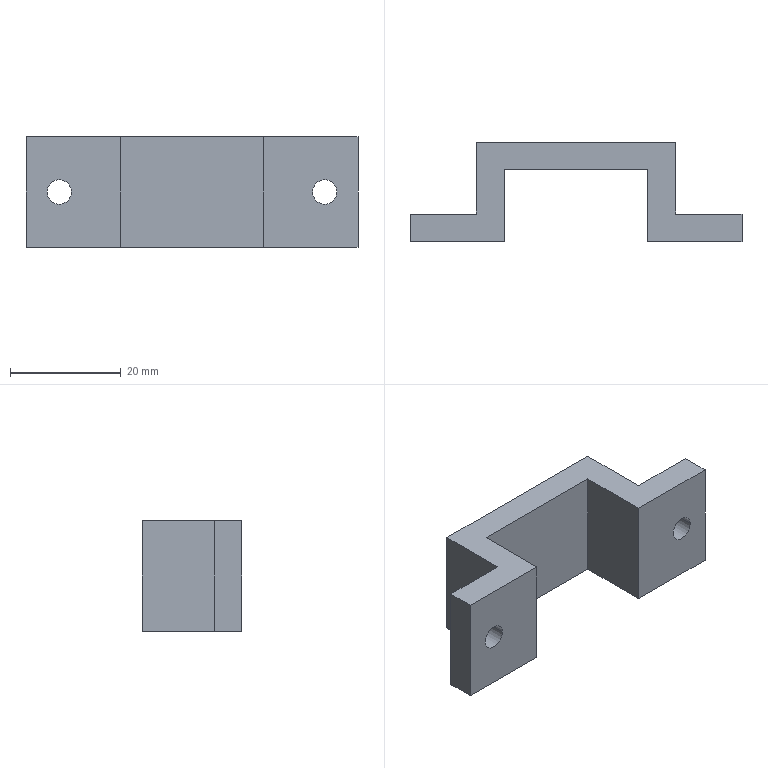Part | SolidWorks | features MirrorStock 1 | 1 solid | 18 faces | box 60 x 18 x 20 mm | volume 8448 mm3 | plane 14 | cylinder 4 | commonest cylinder face diameters 4.4 x4
STEP:
#1=CARTESIAN_POINT('',(51.8,0.,0.));
#2=VERTEX_POINT('',#1);
#3=CARTESIAN_POINT('',(56.2,0.,0.));
#4=VERTEX_POINT('',#3);
#5=CARTESIAN_POINT('',(54.,0.,0.));
#6=DIRECTION('',(0.,-1.,0.));
#7=DIRECTION('',(0.,0.,-1.));
#8=AXIS2_PLACEMENT_3D('',#5,#6,#7);
#9=CIRCLE('',#8,2.2);
#10=EDGE_CURVE('',#2,#4,#9,.T.);
#11=ORIENTED_EDGE('',*,*,#10,.T.);
#12=CARTESIAN_POINT('',(56.2,5.,0.));
#13=VERTEX_POINT('',#12);
#14=CARTESIAN_POINT('',(56.2,-5.,0.));
#15=DIRECTION('',(0.,1.,0.));
#16=VECTOR('',#15,1000.);
#17=LINE('',#14,#16);
#18=EDGE_CURVE('',#4,#13,#17,.T.);
#19=ORIENTED_EDGE('',*,*,#18,.T.);
#20=CARTESIAN_POINT('',(51.8,5.,0.));
#21=VERTEX_POINT('',#20);
#22=CARTESIAN_POINT('',(54.,5.,0.));
#23=DIRECTION('',(0.,-1.,0.));
#24=DIRECTION('',(-1.,0.,0.));
#25=AXIS2_PLACEMENT_3D('',#22,#23,#24);
#26=CIRCLE('',#25,2.2);
#27=EDGE_CURVE('',#21,#13,#26,.T.);
#28=ORIENTED_EDGE('',*,*,#27,.F.);
#29=CARTESIAN_POINT('',(51.8,-5.,0.));
#30=DIRECTION('',(0.,1.,0.));
#31=VECTOR('',#30,1000.);
#32=LINE('',#29,#31);
#33=EDGE_CURVE('',#2,#21,#32,.T.);
#34=ORIENTED_EDGE('',*,*,#33,.F.);
#35=EDGE_LOOP('',(#11,#19,#28,#34));
#36=FACE_OUTER_BOUND('',#35,.T.);
#37=CARTESIAN_POINT('',(54.,-5.,0.));
#38=DIRECTION('',(0.,1.,0.));
#39=DIRECTION('',(-1.,0.,0.));
#40=AXIS2_PLACEMENT_3D('',#37,#38,#39);
#41=CYLINDRICAL_SURFACE('',#40,2.2);
#42=ADVANCED_FACE('',(#36),#41,.F.);
#43=CARTESIAN_POINT('',(3.8,0.,0.));
#44=VERTEX_POINT('',#43);
#45=CARTESIAN_POINT('',(8.2,0.,0.));
#46=VERTEX_POINT('',#45);
#47=CARTESIAN_POINT('',(6.,0.,0.));
#48=DIRECTION('',(0.,-1.,0.));
#49=DIRECTION('',(0.,0.,-1.));
#50=AXIS2_PLACEMENT_3D('',#47,#48,#49);
#51=CIRCLE('',#50,2.2);
#52=EDGE_CURVE('',#44,#46,#51,.T.);
#53=ORIENTED_EDGE('',*,*,#52,.T.);
#54=CARTESIAN_POINT('',(8.2,5.,0.));
#55=VERTEX_POINT('',#54);
#56=CARTESIAN_POINT('',(8.2,-5.,0.));
#57=DIRECTION('',(0.,1.,0.));
#58=VECTOR('',#57,1000.);
#59=LINE('',#56,#58);
#60=EDGE_CURVE('',#46,#55,#59,.T.);
#61=ORIENTED_EDGE('',*,*,#60,.T.);
#62=CARTESIAN_POINT('',(3.8,5.,0.));
#63=VERTEX_POINT('',#62);
#64=CARTESIAN_POINT('',(6.,5.,0.));
#65=DIRECTION('',(0.,-1.,0.));
#66=DIRECTION('',(-1.,0.,0.));
#67=AXIS2_PLACEMENT_3D('',#64,#65,#66);
#68=CIRCLE('',#67,2.2);
#69=EDGE_CURVE('',#63,#55,#68,.T.);
#70=ORIENTED_EDGE('',*,*,#69,.F.);
#71=CARTESIAN_POINT('',(3.8,-5.,0.));
#72=DIRECTION('',(0.,1.,0.));
#73=VECTOR('',#72,1000.);
#74=LINE('',#71,#73);
#75=EDGE_CURVE('',#44,#63,#74,.T.);
#76=ORIENTED_EDGE('',*,*,#75,.F.);
#77=EDGE_LOOP('',(#53,#61,#70,#76));
#78=FACE_OUTER_BOUND('',#77,.T.);
#79=CARTESIAN_POINT('',(6.,-5.,0.));
#80=DIRECTION('',(0.,1.,0.));
#81=DIRECTION('',(-1.,0.,0.));
#82=AXIS2_PLACEMENT_3D('',#79,#80,#81);
#83=CYLINDRICAL_SURFACE('',#82,2.2);
#84=ADVANCED_FACE('',(#78),#83,.F.);
#85=CARTESIAN_POINT('',(0.,5.,10.));
#86=VERTEX_POINT('',#85);
#87=CARTESIAN_POINT('',(0.,0.,10.));
#88=VERTEX_POINT('',#87);
#89=CARTESIAN_POINT('',(0.,5.,10.));
#90=DIRECTION('',(0.,-1.,0.));
#91=VECTOR('',#90,1000.);
#92=LINE('',#89,#91);
#93=EDGE_CURVE('',#86,#88,#92,.T.);
#94=ORIENTED_EDGE('',*,*,#93,.F.);
#95=CARTESIAN_POINT('',(0.,5.,-10.));
#96=VERTEX_POINT('',#95);
#97=CARTESIAN_POINT('',(0.,5.,-10.));
#98=DIRECTION('',(0.,0.,1.));
#99=VECTOR('',#98,1000.);
#100=LINE('',#97,#99);
#101=EDGE_CURVE('',#96,#86,#100,.T.);
#102=ORIENTED_EDGE('',*,*,#101,.F.);
#103=CARTESIAN_POINT('',(0.,0.,-10.));
#104=VERTEX_POINT('',#103);
#105=CARTESIAN_POINT('',(0.,5.,-10.));
#106=DIRECTION('',(0.,-1.,0.));
#107=VECTOR('',#106,1000.);
#108=LINE('',#105,#107);
#109=EDGE_CURVE('',#96,#104,#108,.T.);
#110=ORIENTED_EDGE('',*,*,#109,.T.);
#111=CARTESIAN_POINT('',(0.,0.,-10.));
#112=DIRECTION('',(0.,0.,1.));
#113=VECTOR('',#112,1000.);
#114=LINE('',#111,#113);
#115=EDGE_CURVE('',#104,#88,#114,.T.);
#116=ORIENTED_EDGE('',*,*,#115,.T.);
#117=EDGE_LOOP('',(#94,#102,#110,#116));
#118=FACE_OUTER_BOUND('',#117,.T.);
#119=CARTESIAN_POINT('',(0.,5.,-10.));
#120=DIRECTION('',(1.,0.,0.));
#121=DIRECTION('',(0.,0.,1.));
#122=AXIS2_PLACEMENT_3D('',#119,#120,#121);
#123=PLANE('',#122);
#124=ADVANCED_FACE('',(#118),#123,.F.);
#125=ORIENTED_EDGE('',*,*,#52,.F.);
#126=CARTESIAN_POINT('',(6.,0.,0.));
#127=DIRECTION('',(0.,-1.,0.));
#128=DIRECTION('',(0.,0.,-1.));
#129=AXIS2_PLACEMENT_3D('',#126,#127,#128);
#130=CIRCLE('',#129,2.2);
#131=EDGE_CURVE('',#46,#44,#130,.T.);
#132=ORIENTED_EDGE('',*,*,#131,.F.);
#133=EDGE_LOOP('',(#125,#132));
#134=FACE_BOUND('',#133,.T.);
#135=CARTESIAN_POINT('',(17.,0.,10.));
#136=VERTEX_POINT('',#135);
#137=CARTESIAN_POINT('',(0.,0.,10.));
#138=DIRECTION('',(1.,0.,0.));
#139=VECTOR('',#138,1000.);
#140=LINE('',#137,#139);
#141=EDGE_CURVE('',#88,#136,#140,.T.);
#142=ORIENTED_EDGE('',*,*,#141,.F.);
#143=ORIENTED_EDGE('',*,*,#115,.F.);
#144=CARTESIAN_POINT('',(17.,0.,-10.));
#145=VERTEX_POINT('',#144);
#146=CARTESIAN_POINT('',(0.,0.,-10.));
#147=DIRECTION('',(1.,0.,0.));
#148=VECTOR('',#147,1000.);
#149=LINE('',#146,#148);
#150=EDGE_CURVE('',#104,#145,#149,.T.);
#151=ORIENTED_EDGE('',*,*,#150,.T.);
#152=CARTESIAN_POINT('',(17.,0.,-10.));
#153=DIRECTION('',(0.,0.,1.));
#154=VECTOR('',#153,1000.);
#155=LINE('',#152,#154);
#156=EDGE_CURVE('',#145,#136,#155,.T.);
#157=ORIENTED_EDGE('',*,*,#156,.T.);
#158=EDGE_LOOP('',(#142,#143,#151,#157));
#159=FACE_OUTER_BOUND('',#158,.T.);
#160=CARTESIAN_POINT('',(0.,0.,-10.));
#161=DIRECTION('',(0.,1.,0.));
#162=DIRECTION('',(0.,0.,-1.));
#163=AXIS2_PLACEMENT_3D('',#160,#161,#162);
#164=PLANE('',#163);
#165=ADVANCED_FACE('',(#134,#159),#164,.F.);
#166=CARTESIAN_POINT('',(17.,13.,10.));
#167=VERTEX_POINT('',#166);
#168=CARTESIAN_POINT('',(17.,0.,10.));
#169=DIRECTION('',(0.,1.,0.));
#170=VECTOR('',#169,1000.);
#171=LINE('',#168,#170);
#172=EDGE_CURVE('',#136,#167,#171,.T.);
#173=ORIENTED_EDGE('',*,*,#172,.F.);
#174=ORIENTED_EDGE('',*,*,#156,.F.);
#175=CARTESIAN_POINT('',(17.,13.,-10.));
#176=VERTEX_POINT('',#175);
#177=CARTESIAN_POINT('',(17.,0.,-10.));
#178=DIRECTION('',(0.,1.,0.));
#179=VECTOR('',#178,1000.);
#180=LINE('',#177,#179);
#181=EDGE_CURVE('',#145,#176,#180,.T.);
#182=ORIENTED_EDGE('',*,*,#181,.T.);
#183=CARTESIAN_POINT('',(17.,13.,-10.));
#184=DIRECTION('',(0.,0.,1.));
#185=VECTOR('',#184,1000.);
#186=LINE('',#183,#185);
#187=EDGE_CURVE('',#176,#167,#186,.T.);
#188=ORIENTED_EDGE('',*,*,#187,.T.);
#189=EDGE_LOOP('',(#173,#174,#182,#188));
#190=FACE_OUTER_BOUND('',#189,.T.);
#191=CARTESIAN_POINT('',(17.,0.,-10.));
#192=DIRECTION('',(-1.,0.,0.));
#193=DIRECTION('',(0.,-1.,0.));
#194=AXIS2_PLACEMENT_3D('',#191,#192,#193);
#195=PLANE('',#194);
#196=ADVANCED_FACE('',(#190),#195,.F.);
#197=CARTESIAN_POINT('',(43.,13.,10.));
#198=VERTEX_POINT('',#197);
#199=CARTESIAN_POINT('',(17.,13.,10.));
#200=DIRECTION('',(1.,0.,0.));
#201=VECTOR('',#200,1000.);
#202=LINE('',#199,#201);
#203=EDGE_CURVE('',#167,#198,#202,.T.);
#204=ORIENTED_EDGE('',*,*,#203,.F.);
#205=ORIENTED_EDGE('',*,*,#187,.F.);
#206=CARTESIAN_POINT('',(43.,13.,-10.));
#207=VERTEX_POINT('',#206);
#208=CARTESIAN_POINT('',(17.,13.,-10.));
#209=DIRECTION('',(1.,0.,0.));
#210=VECTOR('',#209,1000.);
#211=LINE('',#208,#210);
#212=EDGE_CURVE('',#176,#207,#211,.T.);
#213=ORIENTED_EDGE('',*,*,#212,.T.);
#214=CARTESIAN_POINT('',(43.,13.,-10.));
#215=DIRECTION('',(0.,0.,1.));
#216=VECTOR('',#215,1000.);
#217=LINE('',#214,#216);
#218=EDGE_CURVE('',#207,#198,#217,.T.);
#219=ORIENTED_EDGE('',*,*,#218,.T.);
#220=EDGE_LOOP('',(#204,#205,#213,#219));
#221=FACE_OUTER_BOUND('',#220,.T.);
#222=CARTESIAN_POINT('',(17.,13.,-10.));
#223=DIRECTION('',(0.,1.,0.));
#224=DIRECTION('',(0.,0.,-1.));
#225=AXIS2_PLACEMENT_3D('',#222,#223,#224);
#226=PLANE('',#225);
#227=ADVANCED_FACE('',(#221),#226,.F.);
#228=CARTESIAN_POINT('',(43.,0.,10.));
#229=VERTEX_POINT('',#228);
#230=CARTESIAN_POINT('',(43.,13.,10.));
#231=DIRECTION('',(0.,-1.,0.));
#232=VECTOR('',#231,1000.);
#233=LINE('',#230,#232);
#234=EDGE_CURVE('',#198,#229,#233,.T.);
#235=ORIENTED_EDGE('',*,*,#234,.F.);
#236=ORIENTED_EDGE('',*,*,#218,.F.);
#237=CARTESIAN_POINT('',(43.,0.,-10.));
#238=VERTEX_POINT('',#237);
#239=CARTESIAN_POINT('',(43.,13.,-10.));
#240=DIRECTION('',(0.,-1.,0.));
#241=VECTOR('',#240,1000.);
#242=LINE('',#239,#241);
#243=EDGE_CURVE('',#207,#238,#242,.T.);
#244=ORIENTED_EDGE('',*,*,#243,.T.);
#245=CARTESIAN_POINT('',(43.,0.,-10.));
#246=DIRECTION('',(0.,0.,1.));
#247=VECTOR('',#246,1000.);
#248=LINE('',#245,#247);
#249=EDGE_CURVE('',#238,#229,#248,.T.);
#250=ORIENTED_EDGE('',*,*,#249,.T.);
#251=EDGE_LOOP('',(#235,#236,#244,#250));
#252=FACE_OUTER_BOUND('',#251,.T.);
#253=CARTESIAN_POINT('',(43.,13.,-10.));
#254=DIRECTION('',(1.,0.,0.));
#255=DIRECTION('',(0.,0.,1.));
#256=AXIS2_PLACEMENT_3D('',#253,#254,#255);
#257=PLANE('',#256);
#258=ADVANCED_FACE('',(#252),#257,.F.);
#259=ORIENTED_EDGE('',*,*,#10,.F.);
#260=CARTESIAN_POINT('',(54.,0.,0.));
#261=DIRECTION('',(0.,-1.,0.));
#262=DIRECTION('',(0.,0.,-1.));
#263=AXIS2_PLACEMENT_3D('',#260,#261,#262);
#264=CIRCLE('',#263,2.2);
#265=EDGE_CURVE('',#4,#2,#264,.T.);
#266=ORIENTED_EDGE('',*,*,#265,.F.);
#267=EDGE_LOOP('',(#259,#266));
#268=FACE_BOUND('',#267,.T.);
#269=CARTESIAN_POINT('',(60.,0.,10.));
#270=VERTEX_POINT('',#269);
#271=CARTESIAN_POINT('',(43.,0.,10.));
#272=DIRECTION('',(1.,0.,0.));
#273=VECTOR('',#272,1000.);
#274=LINE('',#271,#273);
#275=EDGE_CURVE('',#229,#270,#274,.T.);
#276=ORIENTED_EDGE('',*,*,#275,.F.);
#277=ORIENTED_EDGE('',*,*,#249,.F.);
#278=CARTESIAN_POINT('',(60.,0.,-10.));
#279=VERTEX_POINT('',#278);
#280=CARTESIAN_POINT('',(43.,0.,-10.));
#281=DIRECTION('',(1.,0.,0.));
#282=VECTOR('',#281,1000.);
#283=LINE('',#280,#282);
#284=EDGE_CURVE('',#238,#279,#283,.T.);
#285=ORIENTED_EDGE('',*,*,#284,.T.);
#286=CARTESIAN_POINT('',(60.,0.,-10.));
#287=DIRECTION('',(0.,0.,1.));
#288=VECTOR('',#287,1000.);
#289=LINE('',#286,#288);
#290=EDGE_CURVE('',#279,#270,#289,.T.);
#291=ORIENTED_EDGE('',*,*,#290,.T.);
#292=EDGE_LOOP('',(#276,#277,#285,#291));
#293=FACE_OUTER_BOUND('',#292,.T.);
#294=CARTESIAN_POINT('',(43.,0.,-10.));
#295=DIRECTION('',(0.,1.,0.));
#296=DIRECTION('',(0.,0.,-1.));
#297=AXIS2_PLACEMENT_3D('',#294,#295,#296);
#298=PLANE('',#297);
#299=ADVANCED_FACE('',(#268,#293),#298,.F.);
#300=CARTESIAN_POINT('',(60.,5.,10.));
#301=VERTEX_POINT('',#300);
#302=CARTESIAN_POINT('',(60.,0.,10.));
#303=DIRECTION('',(0.,1.,0.));
#304=VECTOR('',#303,1000.);
#305=LINE('',#302,#304);
#306=EDGE_CURVE('',#270,#301,#305,.T.);
#307=ORIENTED_EDGE('',*,*,#306,.F.);
#308=ORIENTED_EDGE('',*,*,#290,.F.);
#309=CARTESIAN_POINT('',(60.,5.,-10.));
#310=VERTEX_POINT('',#309);
#311=CARTESIAN_POINT('',(60.,0.,-10.));
#312=DIRECTION('',(0.,1.,0.));
#313=VECTOR('',#312,1000.);
#314=LINE('',#311,#313);
#315=EDGE_CURVE('',#279,#310,#314,.T.);
#316=ORIENTED_EDGE('',*,*,#315,.T.);
#317=CARTESIAN_POINT('',(60.,5.,-10.));
#318=DIRECTION('',(0.,0.,1.));
#319=VECTOR('',#318,1000.);
#320=LINE('',#317,#319);
#321=EDGE_CURVE('',#310,#301,#320,.T.);
#322=ORIENTED_EDGE('',*,*,#321,.T.);
#323=EDGE_LOOP('',(#307,#308,#316,#322));
#324=FACE_OUTER_BOUND('',#323,.T.);
#325=CARTESIAN_POINT('',(60.,0.,-10.));
#326=DIRECTION('',(-1.,0.,0.));
#327=DIRECTION('',(0.,0.,-1.));
#328=AXIS2_PLACEMENT_3D('',#325,#326,#327);
#329=PLANE('',#328);
#330=ADVANCED_FACE('',(#324),#329,.F.);
#331=ORIENTED_EDGE('',*,*,#27,.T.);
#332=CARTESIAN_POINT('',(54.,5.,0.));
#333=DIRECTION('',(0.,-1.,0.));
#334=DIRECTION('',(-1.,0.,0.));
#335=AXIS2_PLACEMENT_3D('',#332,#333,#334);
#336=CIRCLE('',#335,2.2);
#337=EDGE_CURVE('',#13,#21,#336,.T.);
#338=ORIENTED_EDGE('',*,*,#337,.T.);
#339=EDGE_LOOP('',(#331,#338));
#340=FACE_BOUND('',#339,.T.);
#341=CARTESIAN_POINT('',(48.,5.,10.));
#342=VERTEX_POINT('',#341);
#343=CARTESIAN_POINT('',(60.,5.,10.));
#344=DIRECTION('',(-1.,0.,0.));
#345=VECTOR('',#344,1000.);
#346=LINE('',#343,#345);
#347=EDGE_CURVE('',#301,#342,#346,.T.);
#348=ORIENTED_EDGE('',*,*,#347,.F.);
#349=ORIENTED_EDGE('',*,*,#321,.F.);
#350=CARTESIAN_POINT('',(48.,5.,-10.));
#351=VERTEX_POINT('',#350);
#352=CARTESIAN_POINT('',(60.,5.,-10.));
#353=DIRECTION('',(-1.,0.,0.));
#354=VECTOR('',#353,1000.);
#355=LINE('',#352,#354);
#356=EDGE_CURVE('',#310,#351,#355,.T.);
#357=ORIENTED_EDGE('',*,*,#356,.T.);
#358=CARTESIAN_POINT('',(48.,5.,-10.));
#359=DIRECTION('',(0.,0.,1.));
#360=VECTOR('',#359,1000.);
#361=LINE('',#358,#360);
#362=EDGE_CURVE('',#351,#342,#361,.T.);
#363=ORIENTED_EDGE('',*,*,#362,.T.);
#364=EDGE_LOOP('',(#348,#349,#357,#363));
#365=FACE_OUTER_BOUND('',#364,.T.);
#366=CARTESIAN_POINT('',(60.,5.,-10.));
#367=DIRECTION('',(0.,-1.,0.));
#368=DIRECTION('',(1.,0.,0.));
#369=AXIS2_PLACEMENT_3D('',#366,#367,#368);
#370=PLANE('',#369);
#371=ADVANCED_FACE('',(#340,#365),#370,.F.);
#372=CARTESIAN_POINT('',(48.,18.,10.));
#373=VERTEX_POINT('',#372);
#374=CARTESIAN_POINT('',(48.,5.,10.));
#375=DIRECTION('',(0.,1.,0.));
#376=VECTOR('',#375,1000.);
#377=LINE('',#374,#376);
#378=EDGE_CURVE('',#342,#373,#377,.T.);
#379=ORIENTED_EDGE('',*,*,#378,.F.);
#380=ORIENTED_EDGE('',*,*,#362,.F.);
#381=CARTESIAN_POINT('',(48.,18.,-10.));
#382=VERTEX_POINT('',#381);
#383=CARTESIAN_POINT('',(48.,5.,-10.));
#384=DIRECTION('',(0.,1.,0.));
#385=VECTOR('',#384,1000.);
#386=LINE('',#383,#385);
#387=EDGE_CURVE('',#351,#382,#386,.T.);
#388=ORIENTED_EDGE('',*,*,#387,.T.);
#389=CARTESIAN_POINT('',(48.,18.,-10.));
#390=DIRECTION('',(0.,0.,1.));
#391=VECTOR('',#390,1000.);
#392=LINE('',#389,#391);
#393=EDGE_CURVE('',#382,#373,#392,.T.);
#394=ORIENTED_EDGE('',*,*,#393,.T.);
#395=EDGE_LOOP('',(#379,#380,#388,#394));
#396=FACE_OUTER_BOUND('',#395,.T.);
#397=CARTESIAN_POINT('',(48.,5.,-10.));
#398=DIRECTION('',(-1.,0.,0.));
#399=DIRECTION('',(0.,0.,-1.));
#400=AXIS2_PLACEMENT_3D('',#397,#398,#399);
#401=PLANE('',#400);
#402=ADVANCED_FACE('',(#396),#401,.F.);
#403=CARTESIAN_POINT('',(12.,18.,10.));
#404=VERTEX_POINT('',#403);
#405=CARTESIAN_POINT('',(48.,18.,10.));
#406=DIRECTION('',(-1.,0.,0.));
#407=VECTOR('',#406,1000.);
#408=LINE('',#405,#407);
#409=EDGE_CURVE('',#373,#404,#408,.T.);
#410=ORIENTED_EDGE('',*,*,#409,.F.);
#411=ORIENTED_EDGE('',*,*,#393,.F.);
#412=CARTESIAN_POINT('',(12.,18.,-10.));
#413=VERTEX_POINT('',#412);
#414=CARTESIAN_POINT('',(48.,18.,-10.));
#415=DIRECTION('',(-1.,0.,0.));
#416=VECTOR('',#415,1000.);
#417=LINE('',#414,#416);
#418=EDGE_CURVE('',#382,#413,#417,.T.);
#419=ORIENTED_EDGE('',*,*,#418,.T.);
#420=CARTESIAN_POINT('',(12.,18.,-10.));
#421=DIRECTION('',(0.,0.,1.));
#422=VECTOR('',#421,1000.);
#423=LINE('',#420,#422);
#424=EDGE_CURVE('',#413,#404,#423,.T.);
#425=ORIENTED_EDGE('',*,*,#424,.T.);
#426=EDGE_LOOP('',(#410,#411,#419,#425));
#427=FACE_OUTER_BOUND('',#426,.T.);
#428=CARTESIAN_POINT('',(48.,18.,-10.));
#429=DIRECTION('',(0.,-1.,0.));
#430=DIRECTION('',(1.,0.,0.));
#431=AXIS2_PLACEMENT_3D('',#428,#429,#430);
#432=PLANE('',#431);
#433=ADVANCED_FACE('',(#427),#432,.F.);
#434=CARTESIAN_POINT('',(12.,5.,10.));
#435=VERTEX_POINT('',#434);
#436=CARTESIAN_POINT('',(12.,18.,10.));
#437=DIRECTION('',(0.,-1.,0.));
#438=VECTOR('',#437,1000.);
#439=LINE('',#436,#438);
#440=EDGE_CURVE('',#404,#435,#439,.T.);
#441=ORIENTED_EDGE('',*,*,#440,.F.);
#442=ORIENTED_EDGE('',*,*,#424,.F.);
#443=CARTESIAN_POINT('',(12.,5.,-10.));
#444=VERTEX_POINT('',#443);
#445=CARTESIAN_POINT('',(12.,18.,-10.));
#446=DIRECTION('',(0.,-1.,0.));
#447=VECTOR('',#446,1000.);
#448=LINE('',#445,#447);
#449=EDGE_CURVE('',#413,#444,#448,.T.);
#450=ORIENTED_EDGE('',*,*,#449,.T.);
#451=CARTESIAN_POINT('',(12.,5.,-10.));
#452=DIRECTION('',(0.,0.,1.));
#453=VECTOR('',#452,1000.);
#454=LINE('',#451,#453);
#455=EDGE_CURVE('',#444,#435,#454,.T.);
#456=ORIENTED_EDGE('',*,*,#455,.T.);
#457=EDGE_LOOP('',(#441,#442,#450,#456));
#458=FACE_OUTER_BOUND('',#457,.T.);
#459=CARTESIAN_POINT('',(12.,18.,-10.));
#460=DIRECTION('',(1.,0.,0.));
#461=DIRECTION('',(0.,1.,0.));
#462=AXIS2_PLACEMENT_3D('',#459,#460,#461);
#463=PLANE('',#462);
#464=ADVANCED_FACE('',(#458),#463,.F.);
#465=ORIENTED_EDGE('',*,*,#69,.T.);
#466=CARTESIAN_POINT('',(6.,5.,0.));
#467=DIRECTION('',(0.,-1.,0.));
#468=DIRECTION('',(-1.,0.,0.));
#469=AXIS2_PLACEMENT_3D('',#466,#467,#468);
#470=CIRCLE('',#469,2.2);
#471=EDGE_CURVE('',#55,#63,#470,.T.);
#472=ORIENTED_EDGE('',*,*,#471,.T.);
#473=EDGE_LOOP('',(#465,#472));
#474=FACE_BOUND('',#473,.T.);
#475=CARTESIAN_POINT('',(12.,5.,10.));
#476=DIRECTION('',(-1.,0.,0.));
#477=VECTOR('',#476,1000.);
#478=LINE('',#475,#477);
#479=EDGE_CURVE('',#435,#86,#478,.T.);
#480=ORIENTED_EDGE('',*,*,#479,.F.);
#481=ORIENTED_EDGE('',*,*,#455,.F.);
#482=CARTESIAN_POINT('',(12.,5.,-10.));
#483=DIRECTION('',(-1.,0.,0.));
#484=VECTOR('',#483,1000.);
#485=LINE('',#482,#484);
#486=EDGE_CURVE('',#444,#96,#485,.T.);
#487=ORIENTED_EDGE('',*,*,#486,.T.);
#488=ORIENTED_EDGE('',*,*,#101,.T.);
#489=EDGE_LOOP('',(#480,#481,#487,#488));
#490=FACE_OUTER_BOUND('',#489,.T.);
#491=CARTESIAN_POINT('',(12.,5.,-10.));
#492=DIRECTION('',(0.,-1.,0.));
#493=DIRECTION('',(1.,0.,0.));
#494=AXIS2_PLACEMENT_3D('',#491,#492,#493);
#495=PLANE('',#494);
#496=ADVANCED_FACE('',(#474,#490),#495,.F.);
#497=ORIENTED_EDGE('',*,*,#109,.F.);
#498=ORIENTED_EDGE('',*,*,#486,.F.);
#499=ORIENTED_EDGE('',*,*,#449,.F.);
#500=ORIENTED_EDGE('',*,*,#418,.F.);
#501=ORIENTED_EDGE('',*,*,#387,.F.);
#502=ORIENTED_EDGE('',*,*,#356,.F.);
#503=ORIENTED_EDGE('',*,*,#315,.F.);
#504=ORIENTED_EDGE('',*,*,#284,.F.);
#505=ORIENTED_EDGE('',*,*,#243,.F.);
#506=ORIENTED_EDGE('',*,*,#212,.F.);
#507=ORIENTED_EDGE('',*,*,#181,.F.);
#508=ORIENTED_EDGE('',*,*,#150,.F.);
#509=EDGE_LOOP('',(#497,#498,#499,#500,#501,#502,#503,#504,#505,#506,#507,#508));
#510=FACE_OUTER_BOUND('',#509,.T.);
#511=CARTESIAN_POINT('',(0.,0.,-10.));
#512=DIRECTION('',(0.,0.,-1.));
#513=DIRECTION('',(1.,0.,0.));
#514=AXIS2_PLACEMENT_3D('',#511,#512,#513);
#515=PLANE('',#514);
#516=ADVANCED_FACE('',(#510),#515,.T.);
#517=ORIENTED_EDGE('',*,*,#93,.T.);
#518=ORIENTED_EDGE('',*,*,#141,.T.);
#519=ORIENTED_EDGE('',*,*,#172,.T.);
#520=ORIENTED_EDGE('',*,*,#203,.T.);
#521=ORIENTED_EDGE('',*,*,#234,.T.);
#522=ORIENTED_EDGE('',*,*,#275,.T.);
#523=ORIENTED_EDGE('',*,*,#306,.T.);
#524=ORIENTED_EDGE('',*,*,#347,.T.);
#525=ORIENTED_EDGE('',*,*,#378,.T.);
#526=ORIENTED_EDGE('',*,*,#409,.T.);
#527=ORIENTED_EDGE('',*,*,#440,.T.);
#528=ORIENTED_EDGE('',*,*,#479,.T.);
#529=EDGE_LOOP('',(#517,#518,#519,#520,#521,#522,#523,#524,#525,#526,#527,#528));
#530=FACE_OUTER_BOUND('',#529,.T.);
#531=CARTESIAN_POINT('',(0.,0.,10.));
#532=DIRECTION('',(0.,0.,-1.));
#533=DIRECTION('',(1.,0.,0.));
#534=AXIS2_PLACEMENT_3D('',#531,#532,#533);
#535=PLANE('',#534);
#536=ADVANCED_FACE('',(#530),#535,.F.);
#537=ORIENTED_EDGE('',*,*,#60,.F.);
#538=ORIENTED_EDGE('',*,*,#131,.T.);
#539=ORIENTED_EDGE('',*,*,#75,.T.);
#540=ORIENTED_EDGE('',*,*,#471,.F.);
#541=EDGE_LOOP('',(#537,#538,#539,#540));
#542=FACE_OUTER_BOUND('',#541,.T.);
#543=CARTESIAN_POINT('',(6.,-5.,0.));
#544=DIRECTION('',(0.,1.,0.));
#545=DIRECTION('',(-1.,0.,0.));
#546=AXIS2_PLACEMENT_3D('',#543,#544,#545);
#547=CYLINDRICAL_SURFACE('',#546,2.2);
#548=ADVANCED_FACE('',(#542),#547,.F.);
#549=ORIENTED_EDGE('',*,*,#18,.F.);
#550=ORIENTED_EDGE('',*,*,#265,.T.);
#551=ORIENTED_EDGE('',*,*,#33,.T.);
#552=ORIENTED_EDGE('',*,*,#337,.F.);
#553=EDGE_LOOP('',(#549,#550,#551,#552));
#554=FACE_OUTER_BOUND('',#553,.T.);
#555=CARTESIAN_POINT('',(54.,-5.,0.));
#556=DIRECTION('',(0.,1.,0.));
#557=DIRECTION('',(-1.,0.,0.));
#558=AXIS2_PLACEMENT_3D('',#555,#556,#557);
#559=CYLINDRICAL_SURFACE('',#558,2.2);
#560=ADVANCED_FACE('',(#554),#559,.F.);
#561=CLOSED_SHELL('',(#42,#84,#124,#165,#196,#227,#258,#299,#330,#371,#402,#433,#464,#496,#516,#536,#548,#560));
#562=MANIFOLD_SOLID_BREP('',#561);
#563=CARTESIAN_POINT('',(0.,0.,0.));
#564=DIRECTION('',(0.,0.,1.));
#565=DIRECTION('',(1.,0.,0.));
#566=AXIS2_PLACEMENT_3D('',#563,#564,#565);
#567=(LENGTH_UNIT()NAMED_UNIT(*)SI_UNIT(.MILLI.,.METRE.));
#568=UNCERTAINTY_MEASURE_WITH_UNIT(LENGTH_MEASURE(0.00001),#567,'','');
#569=(NAMED_UNIT(*)PLANE_ANGLE_UNIT()SI_UNIT($,.RADIAN.));
#570=(NAMED_UNIT(*)SI_UNIT($,.STERADIAN.)SOLID_ANGLE_UNIT());
#571=(GEOMETRIC_REPRESENTATION_CONTEXT(3)GLOBAL_UNCERTAINTY_ASSIGNED_CONTEXT((#568))GLOBAL_UNIT_ASSIGNED_CONTEXT((#567,#569,#570))REPRESENTATION_CONTEXT('',''));
#572=ADVANCED_BREP_SHAPE_REPRESENTATION('',(#562,#566),#571);